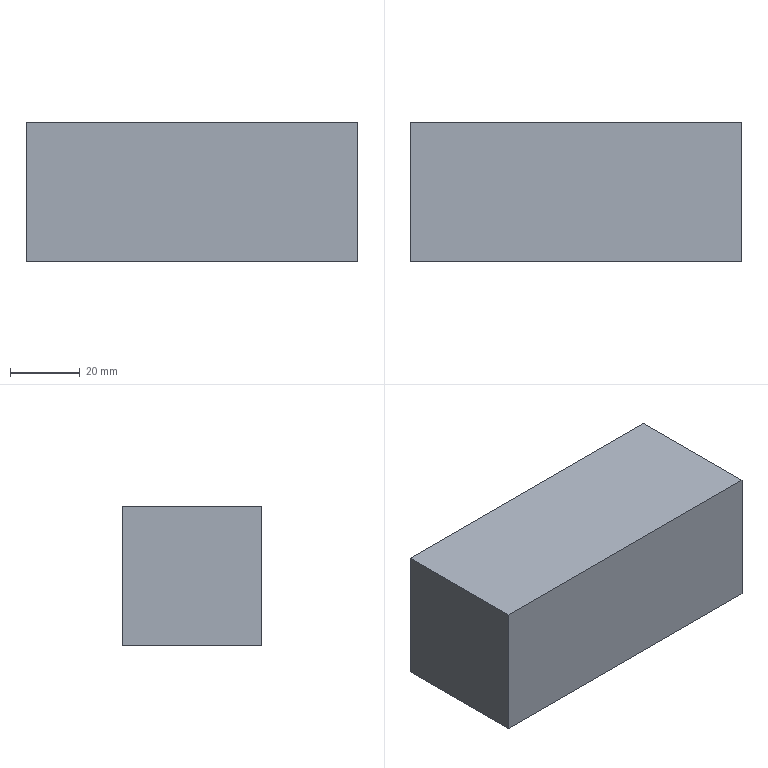Part | STEP file | Spacer block 22 | 1 solid | 6 faces | box 95 x 40 x 40 mm | volume 152000 mm3 | plane 6
STEP:
#1=CARTESIAN_POINT('',(47.5,0.,20.));
#2=VERTEX_POINT('',#1);
#3=CARTESIAN_POINT('',(47.5,0.,-20.));
#4=VERTEX_POINT('',#3);
#5=CARTESIAN_POINT('',(47.5,0.,-20.));
#6=DIRECTION('',(0.,0.,-1.));
#7=VECTOR('',#6,1000.);
#8=LINE('',#5,#7);
#9=EDGE_CURVE('',#2,#4,#8,.T.);
#10=ORIENTED_EDGE('',*,*,#9,.T.);
#11=CARTESIAN_POINT('',(47.5,40.,-20.));
#12=VERTEX_POINT('',#11);
#13=CARTESIAN_POINT('',(47.5,40.,-20.));
#14=DIRECTION('',(0.,-1.,0.));
#15=VECTOR('',#14,1000.);
#16=LINE('',#13,#15);
#17=EDGE_CURVE('',#12,#4,#16,.T.);
#18=ORIENTED_EDGE('',*,*,#17,.F.);
#19=CARTESIAN_POINT('',(47.5,40.,20.));
#20=VERTEX_POINT('',#19);
#21=CARTESIAN_POINT('',(47.5,40.,-20.));
#22=DIRECTION('',(0.,0.,-1.));
#23=VECTOR('',#22,1000.);
#24=LINE('',#21,#23);
#25=EDGE_CURVE('',#20,#12,#24,.T.);
#26=ORIENTED_EDGE('',*,*,#25,.F.);
#27=CARTESIAN_POINT('',(47.5,40.,20.));
#28=DIRECTION('',(0.,-1.,0.));
#29=VECTOR('',#28,1000.);
#30=LINE('',#27,#29);
#31=EDGE_CURVE('',#20,#2,#30,.T.);
#32=ORIENTED_EDGE('',*,*,#31,.T.);
#33=EDGE_LOOP('',(#10,#18,#26,#32));
#34=FACE_OUTER_BOUND('',#33,.T.);
#35=CARTESIAN_POINT('',(47.5,40.,-20.));
#36=DIRECTION('',(-1.,0.,0.));
#37=DIRECTION('',(0.,0.,1.));
#38=AXIS2_PLACEMENT_3D('',#35,#36,#37);
#39=PLANE('',#38);
#40=ADVANCED_FACE('',(#34),#39,.F.);
#41=CARTESIAN_POINT('',(-47.5,0.,-20.));
#42=VERTEX_POINT('',#41);
#43=CARTESIAN_POINT('',(-47.5,0.,-20.));
#44=DIRECTION('',(-1.,0.,0.));
#45=VECTOR('',#44,1000.);
#46=LINE('',#43,#45);
#47=EDGE_CURVE('',#4,#42,#46,.T.);
#48=ORIENTED_EDGE('',*,*,#47,.T.);
#49=CARTESIAN_POINT('',(-47.5,40.,-20.));
#50=VERTEX_POINT('',#49);
#51=CARTESIAN_POINT('',(-47.5,40.,-20.));
#52=DIRECTION('',(0.,-1.,0.));
#53=VECTOR('',#52,1000.);
#54=LINE('',#51,#53);
#55=EDGE_CURVE('',#50,#42,#54,.T.);
#56=ORIENTED_EDGE('',*,*,#55,.F.);
#57=CARTESIAN_POINT('',(-47.5,40.,-20.));
#58=DIRECTION('',(-1.,0.,0.));
#59=VECTOR('',#58,1000.);
#60=LINE('',#57,#59);
#61=EDGE_CURVE('',#12,#50,#60,.T.);
#62=ORIENTED_EDGE('',*,*,#61,.F.);
#63=ORIENTED_EDGE('',*,*,#17,.T.);
#64=EDGE_LOOP('',(#48,#56,#62,#63));
#65=FACE_OUTER_BOUND('',#64,.T.);
#66=CARTESIAN_POINT('',(-47.5,40.,-20.));
#67=DIRECTION('',(0.,0.,1.));
#68=DIRECTION('',(1.,0.,0.));
#69=AXIS2_PLACEMENT_3D('',#66,#67,#68);
#70=PLANE('',#69);
#71=ADVANCED_FACE('',(#65),#70,.F.);
#72=CARTESIAN_POINT('',(-47.5,0.,20.));
#73=VERTEX_POINT('',#72);
#74=CARTESIAN_POINT('',(-47.5,0.,-20.));
#75=DIRECTION('',(0.,0.,1.));
#76=VECTOR('',#75,1000.);
#77=LINE('',#74,#76);
#78=EDGE_CURVE('',#42,#73,#77,.T.);
#79=ORIENTED_EDGE('',*,*,#78,.T.);
#80=CARTESIAN_POINT('',(-47.5,40.,20.));
#81=VERTEX_POINT('',#80);
#82=CARTESIAN_POINT('',(-47.5,40.,20.));
#83=DIRECTION('',(0.,-1.,0.));
#84=VECTOR('',#83,1000.);
#85=LINE('',#82,#84);
#86=EDGE_CURVE('',#81,#73,#85,.T.);
#87=ORIENTED_EDGE('',*,*,#86,.F.);
#88=CARTESIAN_POINT('',(-47.5,40.,-20.));
#89=DIRECTION('',(0.,0.,1.));
#90=VECTOR('',#89,1000.);
#91=LINE('',#88,#90);
#92=EDGE_CURVE('',#50,#81,#91,.T.);
#93=ORIENTED_EDGE('',*,*,#92,.F.);
#94=ORIENTED_EDGE('',*,*,#55,.T.);
#95=EDGE_LOOP('',(#79,#87,#93,#94));
#96=FACE_OUTER_BOUND('',#95,.T.);
#97=CARTESIAN_POINT('',(-47.5,40.,-20.));
#98=DIRECTION('',(1.,0.,0.));
#99=DIRECTION('',(0.,0.,-1.));
#100=AXIS2_PLACEMENT_3D('',#97,#98,#99);
#101=PLANE('',#100);
#102=ADVANCED_FACE('',(#96),#101,.F.);
#103=CARTESIAN_POINT('',(-47.5,0.,20.));
#104=DIRECTION('',(1.,0.,0.));
#105=VECTOR('',#104,1000.);
#106=LINE('',#103,#105);
#107=EDGE_CURVE('',#73,#2,#106,.T.);
#108=ORIENTED_EDGE('',*,*,#107,.T.);
#109=ORIENTED_EDGE('',*,*,#31,.F.);
#110=CARTESIAN_POINT('',(-47.5,40.,20.));
#111=DIRECTION('',(1.,0.,0.));
#112=VECTOR('',#111,1000.);
#113=LINE('',#110,#112);
#114=EDGE_CURVE('',#81,#20,#113,.T.);
#115=ORIENTED_EDGE('',*,*,#114,.F.);
#116=ORIENTED_EDGE('',*,*,#86,.T.);
#117=EDGE_LOOP('',(#108,#109,#115,#116));
#118=FACE_OUTER_BOUND('',#117,.T.);
#119=CARTESIAN_POINT('',(-47.5,40.,20.));
#120=DIRECTION('',(0.,0.,-1.));
#121=DIRECTION('',(-1.,0.,0.));
#122=AXIS2_PLACEMENT_3D('',#119,#120,#121);
#123=PLANE('',#122);
#124=ADVANCED_FACE('',(#118),#123,.F.);
#125=ORIENTED_EDGE('',*,*,#25,.T.);
#126=ORIENTED_EDGE('',*,*,#61,.T.);
#127=ORIENTED_EDGE('',*,*,#92,.T.);
#128=ORIENTED_EDGE('',*,*,#114,.T.);
#129=EDGE_LOOP('',(#125,#126,#127,#128));
#130=FACE_OUTER_BOUND('',#129,.T.);
#131=CARTESIAN_POINT('',(0.,40.,0.));
#132=DIRECTION('',(0.,1.,0.));
#133=DIRECTION('',(0.,0.,1.));
#134=AXIS2_PLACEMENT_3D('',#131,#132,#133);
#135=PLANE('',#134);
#136=ADVANCED_FACE('',(#130),#135,.T.);
#137=ORIENTED_EDGE('',*,*,#9,.F.);
#138=ORIENTED_EDGE('',*,*,#107,.F.);
#139=ORIENTED_EDGE('',*,*,#78,.F.);
#140=ORIENTED_EDGE('',*,*,#47,.F.);
#141=EDGE_LOOP('',(#137,#138,#139,#140));
#142=FACE_OUTER_BOUND('',#141,.T.);
#143=CARTESIAN_POINT('',(0.,0.,0.));
#144=DIRECTION('',(0.,1.,0.));
#145=DIRECTION('',(0.,0.,1.));
#146=AXIS2_PLACEMENT_3D('',#143,#144,#145);
#147=PLANE('',#146);
#148=ADVANCED_FACE('',(#142),#147,.F.);
#149=CLOSED_SHELL('',(#40,#71,#102,#124,#136,#148));
#150=MANIFOLD_SOLID_BREP('',#149);
#151=CARTESIAN_POINT('',(0.,0.,0.));
#152=DIRECTION('',(0.,0.,1.));
#153=DIRECTION('',(1.,0.,0.));
#154=AXIS2_PLACEMENT_3D('',#151,#152,#153);
#155=(LENGTH_UNIT()NAMED_UNIT(*)SI_UNIT(.MILLI.,.METRE.));
#156=UNCERTAINTY_MEASURE_WITH_UNIT(LENGTH_MEASURE(0.00001),#155,'','');
#157=(NAMED_UNIT(*)PLANE_ANGLE_UNIT()SI_UNIT($,.RADIAN.));
#158=(NAMED_UNIT(*)SI_UNIT($,.STERADIAN.)SOLID_ANGLE_UNIT());
#159=(GEOMETRIC_REPRESENTATION_CONTEXT(3)GLOBAL_UNCERTAINTY_ASSIGNED_CONTEXT((#156))GLOBAL_UNIT_ASSIGNED_CONTEXT((#155,#157,#158))REPRESENTATION_CONTEXT('',''));
#160=ADVANCED_BREP_SHAPE_REPRESENTATION('',(#150,#154),#159);